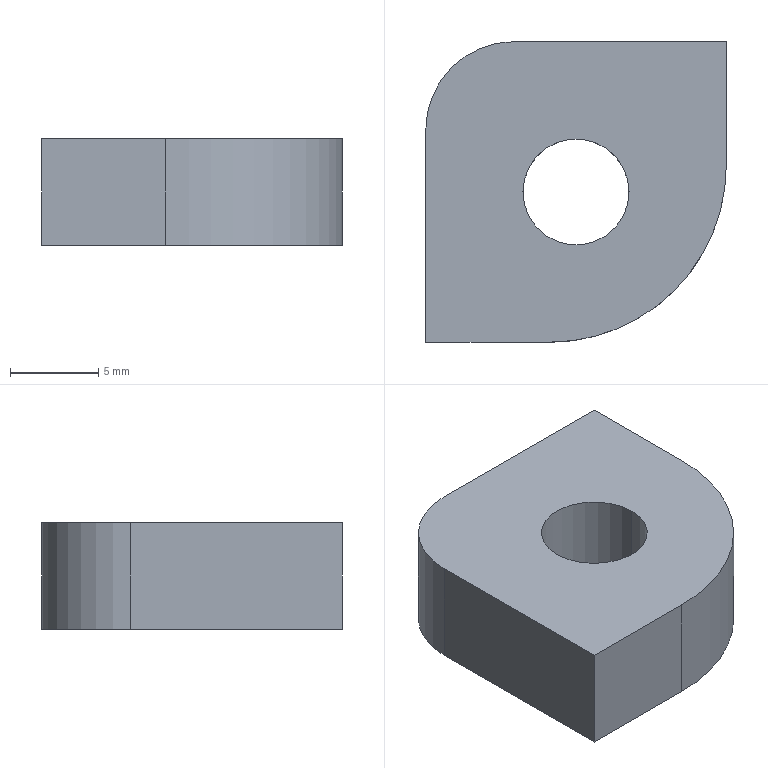Part | SolidWorks | features Fillet 2, Extrusion 1, ICE 1 | 1 solid | 10 faces | box 17 x 17 x 6 mm | volume 1403 mm3 | plane 6 | cylinder 4 | commonest cylinder face diameters 6 x2 10 x1 20 x1
STEP:
#1=CARTESIAN_POINT('',(5.5,-8.5,0.));
#2=VERTEX_POINT('',#1);
#3=CARTESIAN_POINT('',(11.5,-8.5,0.));
#4=VERTEX_POINT('',#3);
#5=CARTESIAN_POINT('',(8.5,-8.5,0.));
#6=DIRECTION('',(0.,0.,1.));
#7=DIRECTION('',(1.,0.,0.));
#8=AXIS2_PLACEMENT_3D('',#5,#6,#7);
#9=CIRCLE('',#8,3.);
#10=EDGE_CURVE('',#2,#4,#9,.T.);
#11=ORIENTED_EDGE('',*,*,#10,.F.);
#12=CARTESIAN_POINT('',(5.5,-8.5,6.));
#13=VERTEX_POINT('',#12);
#14=CARTESIAN_POINT('',(5.5,-8.5,0.));
#15=DIRECTION('',(0.,0.,1.));
#16=VECTOR('',#15,1000.);
#17=LINE('',#14,#16);
#18=EDGE_CURVE('',#2,#13,#17,.T.);
#19=ORIENTED_EDGE('',*,*,#18,.T.);
#20=CARTESIAN_POINT('',(11.5,-8.5,6.));
#21=VERTEX_POINT('',#20);
#22=CARTESIAN_POINT('',(8.5,-8.5,6.));
#23=DIRECTION('',(0.,0.,1.));
#24=DIRECTION('',(1.,0.,0.));
#25=AXIS2_PLACEMENT_3D('',#22,#23,#24);
#26=CIRCLE('',#25,3.);
#27=EDGE_CURVE('',#13,#21,#26,.T.);
#28=ORIENTED_EDGE('',*,*,#27,.T.);
#29=CARTESIAN_POINT('',(11.5,-8.5,0.));
#30=DIRECTION('',(0.,0.,1.));
#31=VECTOR('',#30,1000.);
#32=LINE('',#29,#31);
#33=EDGE_CURVE('',#4,#21,#32,.T.);
#34=ORIENTED_EDGE('',*,*,#33,.F.);
#35=EDGE_LOOP('',(#11,#19,#28,#34));
#36=FACE_OUTER_BOUND('',#35,.T.);
#37=CARTESIAN_POINT('',(8.5,-8.5,0.));
#38=DIRECTION('',(0.,0.,1.));
#39=DIRECTION('',(1.,0.,0.));
#40=AXIS2_PLACEMENT_3D('',#37,#38,#39);
#41=CYLINDRICAL_SURFACE('',#40,3.);
#42=ADVANCED_FACE('',(#36),#41,.F.);
#43=CARTESIAN_POINT('',(0.,-5.,6.));
#44=VERTEX_POINT('',#43);
#45=CARTESIAN_POINT('',(0.,-17.,6.));
#46=VERTEX_POINT('',#45);
#47=CARTESIAN_POINT('',(0.,0.,6.));
#48=DIRECTION('',(0.,-1.,0.));
#49=VECTOR('',#48,1000.);
#50=LINE('',#47,#49);
#51=EDGE_CURVE('',#44,#46,#50,.T.);
#52=ORIENTED_EDGE('',*,*,#51,.F.);
#53=CARTESIAN_POINT('',(0.,-5.,0.));
#54=VERTEX_POINT('',#53);
#55=CARTESIAN_POINT('',(0.,-5.,6.));
#56=DIRECTION('',(0.,0.,-1.));
#57=VECTOR('',#56,1000.);
#58=LINE('',#55,#57);
#59=EDGE_CURVE('',#44,#54,#58,.T.);
#60=ORIENTED_EDGE('',*,*,#59,.T.);
#61=CARTESIAN_POINT('',(0.,-17.,0.));
#62=VERTEX_POINT('',#61);
#63=CARTESIAN_POINT('',(0.,0.,0.));
#64=DIRECTION('',(0.,-1.,0.));
#65=VECTOR('',#64,1000.);
#66=LINE('',#63,#65);
#67=EDGE_CURVE('',#54,#62,#66,.T.);
#68=ORIENTED_EDGE('',*,*,#67,.T.);
#69=CARTESIAN_POINT('',(0.,-17.,6.));
#70=DIRECTION('',(0.,0.,-1.));
#71=VECTOR('',#70,1000.);
#72=LINE('',#69,#71);
#73=EDGE_CURVE('',#46,#62,#72,.T.);
#74=ORIENTED_EDGE('',*,*,#73,.F.);
#75=EDGE_LOOP('',(#52,#60,#68,#74));
#76=FACE_OUTER_BOUND('',#75,.T.);
#77=CARTESIAN_POINT('',(0.,0.,6.));
#78=DIRECTION('',(1.,0.,0.));
#79=DIRECTION('',(0.,1.,0.));
#80=AXIS2_PLACEMENT_3D('',#77,#78,#79);
#81=PLANE('',#80);
#82=ADVANCED_FACE('',(#76),#81,.F.);
#83=CARTESIAN_POINT('',(7.,-17.,0.));
#84=VERTEX_POINT('',#83);
#85=CARTESIAN_POINT('',(0.,-17.,0.));
#86=DIRECTION('',(1.,0.,0.));
#87=VECTOR('',#86,1000.);
#88=LINE('',#85,#87);
#89=EDGE_CURVE('',#62,#84,#88,.T.);
#90=ORIENTED_EDGE('',*,*,#89,.T.);
#91=CARTESIAN_POINT('',(7.,-17.,6.));
#92=VERTEX_POINT('',#91);
#93=CARTESIAN_POINT('',(7.,-17.,6.));
#94=DIRECTION('',(0.,0.,1.));
#95=VECTOR('',#94,1000.);
#96=LINE('',#93,#95);
#97=EDGE_CURVE('',#84,#92,#96,.T.);
#98=ORIENTED_EDGE('',*,*,#97,.T.);
#99=CARTESIAN_POINT('',(0.,-17.,6.));
#100=DIRECTION('',(1.,0.,0.));
#101=VECTOR('',#100,1000.);
#102=LINE('',#99,#101);
#103=EDGE_CURVE('',#46,#92,#102,.T.);
#104=ORIENTED_EDGE('',*,*,#103,.F.);
#105=ORIENTED_EDGE('',*,*,#73,.T.);
#106=EDGE_LOOP('',(#90,#98,#104,#105));
#107=FACE_OUTER_BOUND('',#106,.T.);
#108=CARTESIAN_POINT('',(0.,-17.,6.));
#109=DIRECTION('',(0.,1.,0.));
#110=DIRECTION('',(0.,0.,1.));
#111=AXIS2_PLACEMENT_3D('',#108,#109,#110);
#112=PLANE('',#111);
#113=ADVANCED_FACE('',(#107),#112,.F.);
#114=CARTESIAN_POINT('',(17.,-7.,6.));
#115=VERTEX_POINT('',#114);
#116=CARTESIAN_POINT('',(17.,0.,6.));
#117=VERTEX_POINT('',#116);
#118=CARTESIAN_POINT('',(17.,0.,6.));
#119=DIRECTION('',(0.,1.,0.));
#120=VECTOR('',#119,1000.);
#121=LINE('',#118,#120);
#122=EDGE_CURVE('',#115,#117,#121,.T.);
#123=ORIENTED_EDGE('',*,*,#122,.F.);
#124=CARTESIAN_POINT('',(17.,-7.,0.));
#125=VERTEX_POINT('',#124);
#126=CARTESIAN_POINT('',(17.,-7.,6.));
#127=DIRECTION('',(0.,0.,-1.));
#128=VECTOR('',#127,1000.);
#129=LINE('',#126,#128);
#130=EDGE_CURVE('',#115,#125,#129,.T.);
#131=ORIENTED_EDGE('',*,*,#130,.T.);
#132=CARTESIAN_POINT('',(17.,0.,0.));
#133=VERTEX_POINT('',#132);
#134=CARTESIAN_POINT('',(17.,0.,0.));
#135=DIRECTION('',(0.,1.,0.));
#136=VECTOR('',#135,1000.);
#137=LINE('',#134,#136);
#138=EDGE_CURVE('',#125,#133,#137,.T.);
#139=ORIENTED_EDGE('',*,*,#138,.T.);
#140=CARTESIAN_POINT('',(17.,0.,6.));
#141=DIRECTION('',(0.,0.,-1.));
#142=VECTOR('',#141,1000.);
#143=LINE('',#140,#142);
#144=EDGE_CURVE('',#117,#133,#143,.T.);
#145=ORIENTED_EDGE('',*,*,#144,.F.);
#146=EDGE_LOOP('',(#123,#131,#139,#145));
#147=FACE_OUTER_BOUND('',#146,.T.);
#148=CARTESIAN_POINT('',(17.,0.,6.));
#149=DIRECTION('',(-1.,0.,0.));
#150=DIRECTION('',(0.,-1.,0.));
#151=AXIS2_PLACEMENT_3D('',#148,#149,#150);
#152=PLANE('',#151);
#153=ADVANCED_FACE('',(#147),#152,.F.);
#154=CARTESIAN_POINT('',(5.,0.,0.));
#155=VERTEX_POINT('',#154);
#156=CARTESIAN_POINT('',(0.,0.,0.));
#157=DIRECTION('',(-1.,0.,0.));
#158=VECTOR('',#157,1000.);
#159=LINE('',#156,#158);
#160=EDGE_CURVE('',#133,#155,#159,.T.);
#161=ORIENTED_EDGE('',*,*,#160,.T.);
#162=CARTESIAN_POINT('',(5.,0.,6.));
#163=VERTEX_POINT('',#162);
#164=CARTESIAN_POINT('',(5.,0.,6.));
#165=DIRECTION('',(0.,0.,1.));
#166=VECTOR('',#165,1000.);
#167=LINE('',#164,#166);
#168=EDGE_CURVE('',#155,#163,#167,.T.);
#169=ORIENTED_EDGE('',*,*,#168,.T.);
#170=CARTESIAN_POINT('',(0.,0.,6.));
#171=DIRECTION('',(-1.,0.,0.));
#172=VECTOR('',#171,1000.);
#173=LINE('',#170,#172);
#174=EDGE_CURVE('',#117,#163,#173,.T.);
#175=ORIENTED_EDGE('',*,*,#174,.F.);
#176=ORIENTED_EDGE('',*,*,#144,.T.);
#177=EDGE_LOOP('',(#161,#169,#175,#176));
#178=FACE_OUTER_BOUND('',#177,.T.);
#179=CARTESIAN_POINT('',(0.,0.,6.));
#180=DIRECTION('',(0.,-1.,0.));
#181=DIRECTION('',(0.,0.,-1.));
#182=AXIS2_PLACEMENT_3D('',#179,#180,#181);
#183=PLANE('',#182);
#184=ADVANCED_FACE('',(#178),#183,.F.);
#185=CARTESIAN_POINT('',(8.5,-8.5,6.));
#186=DIRECTION('',(0.,0.,1.));
#187=DIRECTION('',(1.,0.,0.));
#188=AXIS2_PLACEMENT_3D('',#185,#186,#187);
#189=CIRCLE('',#188,3.);
#190=EDGE_CURVE('',#21,#13,#189,.T.);
#191=ORIENTED_EDGE('',*,*,#190,.F.);
#192=ORIENTED_EDGE('',*,*,#27,.F.);
#193=EDGE_LOOP('',(#191,#192));
#194=FACE_BOUND('',#193,.T.);
#195=ORIENTED_EDGE('',*,*,#174,.T.);
#196=CARTESIAN_POINT('',(5.,-5.,6.));
#197=DIRECTION('',(0.,0.,1.));
#198=DIRECTION('',(1.,0.,0.));
#199=AXIS2_PLACEMENT_3D('',#196,#197,#198);
#200=CIRCLE('',#199,5.);
#201=EDGE_CURVE('',#163,#44,#200,.T.);
#202=ORIENTED_EDGE('',*,*,#201,.T.);
#203=ORIENTED_EDGE('',*,*,#51,.T.);
#204=ORIENTED_EDGE('',*,*,#103,.T.);
#205=CARTESIAN_POINT('',(7.,-7.,6.));
#206=DIRECTION('',(0.,0.,1.));
#207=DIRECTION('',(1.,0.,0.));
#208=AXIS2_PLACEMENT_3D('',#205,#206,#207);
#209=CIRCLE('',#208,10.);
#210=EDGE_CURVE('',#92,#115,#209,.T.);
#211=ORIENTED_EDGE('',*,*,#210,.T.);
#212=ORIENTED_EDGE('',*,*,#122,.T.);
#213=EDGE_LOOP('',(#195,#202,#203,#204,#211,#212));
#214=FACE_OUTER_BOUND('',#213,.T.);
#215=CARTESIAN_POINT('',(0.,0.,6.));
#216=DIRECTION('',(0.,0.,1.));
#217=DIRECTION('',(1.,0.,0.));
#218=AXIS2_PLACEMENT_3D('',#215,#216,#217);
#219=PLANE('',#218);
#220=ADVANCED_FACE('',(#194,#214),#219,.T.);
#221=CARTESIAN_POINT('',(8.5,-8.5,0.));
#222=DIRECTION('',(0.,0.,1.));
#223=DIRECTION('',(1.,0.,0.));
#224=AXIS2_PLACEMENT_3D('',#221,#222,#223);
#225=CIRCLE('',#224,3.);
#226=EDGE_CURVE('',#4,#2,#225,.T.);
#227=ORIENTED_EDGE('',*,*,#226,.T.);
#228=ORIENTED_EDGE('',*,*,#10,.T.);
#229=EDGE_LOOP('',(#227,#228));
#230=FACE_BOUND('',#229,.T.);
#231=ORIENTED_EDGE('',*,*,#67,.F.);
#232=CARTESIAN_POINT('',(5.,-5.,0.));
#233=DIRECTION('',(0.,0.,-1.));
#234=DIRECTION('',(1.,0.,0.));
#235=AXIS2_PLACEMENT_3D('',#232,#233,#234);
#236=CIRCLE('',#235,5.);
#237=EDGE_CURVE('',#54,#155,#236,.T.);
#238=ORIENTED_EDGE('',*,*,#237,.T.);
#239=ORIENTED_EDGE('',*,*,#160,.F.);
#240=ORIENTED_EDGE('',*,*,#138,.F.);
#241=CARTESIAN_POINT('',(7.,-7.,0.));
#242=DIRECTION('',(0.,0.,-1.));
#243=DIRECTION('',(1.,0.,0.));
#244=AXIS2_PLACEMENT_3D('',#241,#242,#243);
#245=CIRCLE('',#244,10.);
#246=EDGE_CURVE('',#125,#84,#245,.T.);
#247=ORIENTED_EDGE('',*,*,#246,.T.);
#248=ORIENTED_EDGE('',*,*,#89,.F.);
#249=EDGE_LOOP('',(#231,#238,#239,#240,#247,#248));
#250=FACE_OUTER_BOUND('',#249,.T.);
#251=CARTESIAN_POINT('',(0.,0.,0.));
#252=DIRECTION('',(0.,0.,1.));
#253=DIRECTION('',(1.,0.,0.));
#254=AXIS2_PLACEMENT_3D('',#251,#252,#253);
#255=PLANE('',#254);
#256=ADVANCED_FACE('',(#230,#250),#255,.F.);
#257=ORIENTED_EDGE('',*,*,#210,.F.);
#258=ORIENTED_EDGE('',*,*,#97,.F.);
#259=ORIENTED_EDGE('',*,*,#246,.F.);
#260=ORIENTED_EDGE('',*,*,#130,.F.);
#261=EDGE_LOOP('',(#257,#258,#259,#260));
#262=FACE_OUTER_BOUND('',#261,.T.);
#263=CARTESIAN_POINT('',(7.,-7.,6.));
#264=DIRECTION('',(0.,0.,-1.));
#265=DIRECTION('',(-1.,0.,0.));
#266=AXIS2_PLACEMENT_3D('',#263,#264,#265);
#267=CYLINDRICAL_SURFACE('',#266,10.);
#268=ADVANCED_FACE('',(#262),#267,.T.);
#269=ORIENTED_EDGE('',*,*,#201,.F.);
#270=ORIENTED_EDGE('',*,*,#168,.F.);
#271=ORIENTED_EDGE('',*,*,#237,.F.);
#272=ORIENTED_EDGE('',*,*,#59,.F.);
#273=EDGE_LOOP('',(#269,#270,#271,#272));
#274=FACE_OUTER_BOUND('',#273,.T.);
#275=CARTESIAN_POINT('',(5.,-5.,6.));
#276=DIRECTION('',(0.,0.,-1.));
#277=DIRECTION('',(-1.,0.,0.));
#278=AXIS2_PLACEMENT_3D('',#275,#276,#277);
#279=CYLINDRICAL_SURFACE('',#278,5.);
#280=ADVANCED_FACE('',(#274),#279,.T.);
#281=ORIENTED_EDGE('',*,*,#18,.F.);
#282=ORIENTED_EDGE('',*,*,#226,.F.);
#283=ORIENTED_EDGE('',*,*,#33,.T.);
#284=ORIENTED_EDGE('',*,*,#190,.T.);
#285=EDGE_LOOP('',(#281,#282,#283,#284));
#286=FACE_OUTER_BOUND('',#285,.T.);
#287=CARTESIAN_POINT('',(8.5,-8.5,0.));
#288=DIRECTION('',(0.,0.,1.));
#289=DIRECTION('',(1.,0.,0.));
#290=AXIS2_PLACEMENT_3D('',#287,#288,#289);
#291=CYLINDRICAL_SURFACE('',#290,3.);
#292=ADVANCED_FACE('',(#286),#291,.F.);
#293=CLOSED_SHELL('',(#42,#82,#113,#153,#184,#220,#256,#268,#280,#292));
#294=MANIFOLD_SOLID_BREP('',#293);
#295=CARTESIAN_POINT('',(0.,0.,0.));
#296=DIRECTION('',(0.,0.,1.));
#297=DIRECTION('',(1.,0.,0.));
#298=AXIS2_PLACEMENT_3D('',#295,#296,#297);
#299=(LENGTH_UNIT()NAMED_UNIT(*)SI_UNIT(.MILLI.,.METRE.));
#300=UNCERTAINTY_MEASURE_WITH_UNIT(LENGTH_MEASURE(0.00001),#299,'','');
#301=(NAMED_UNIT(*)PLANE_ANGLE_UNIT()SI_UNIT($,.RADIAN.));
#302=(NAMED_UNIT(*)SI_UNIT($,.STERADIAN.)SOLID_ANGLE_UNIT());
#303=(GEOMETRIC_REPRESENTATION_CONTEXT(3)GLOBAL_UNCERTAINTY_ASSIGNED_CONTEXT((#300))GLOBAL_UNIT_ASSIGNED_CONTEXT((#299,#301,#302))REPRESENTATION_CONTEXT('',''));
#304=ADVANCED_BREP_SHAPE_REPRESENTATION('',(#294,#298),#303);